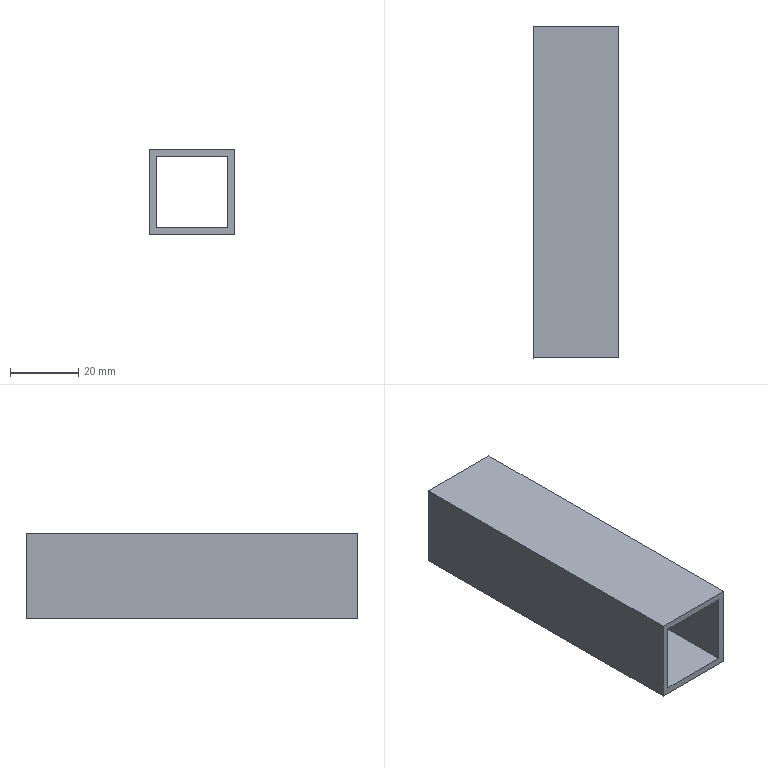Part | NX | features solid 2 | 1 solid | 10 faces | box 25 x 97 x 25 mm | volume 17848 mm3 | plane 10
STEP:
#1=CARTESIAN_POINT('',(-97.5,-106.5,-75.));
#2=VERTEX_POINT('',#1);
#3=CARTESIAN_POINT('',(-97.5,-203.5,-75.));
#4=VERTEX_POINT('',#3);
#5=CARTESIAN_POINT('',(-97.5,-125.,-75.));
#6=DIRECTION('',(0.,-1.,0.));
#7=VECTOR('',#6,1000.);
#8=LINE('',#5,#7);
#9=EDGE_CURVE('',#2,#4,#8,.T.);
#10=ORIENTED_EDGE('',*,*,#9,.T.);
#11=CARTESIAN_POINT('',(-122.5,-203.5,-75.));
#12=VERTEX_POINT('',#11);
#13=CARTESIAN_POINT('',(-95.,-203.5,-75.));
#14=DIRECTION('',(-1.,0.,0.));
#15=VECTOR('',#14,1000.);
#16=LINE('',#13,#15);
#17=EDGE_CURVE('',#4,#12,#16,.T.);
#18=ORIENTED_EDGE('',*,*,#17,.T.);
#19=CARTESIAN_POINT('',(-122.5,-106.5,-75.));
#20=VERTEX_POINT('',#19);
#21=CARTESIAN_POINT('',(-122.5,-125.,-75.));
#22=DIRECTION('',(0.,-1.,0.));
#23=VECTOR('',#22,1000.);
#24=LINE('',#21,#23);
#25=EDGE_CURVE('',#20,#12,#24,.T.);
#26=ORIENTED_EDGE('',*,*,#25,.F.);
#27=CARTESIAN_POINT('',(-95.,-106.5,-75.));
#28=DIRECTION('',(1.,0.,0.));
#29=VECTOR('',#28,1000.);
#30=LINE('',#27,#29);
#31=EDGE_CURVE('',#2,#20,#30,.F.);
#32=ORIENTED_EDGE('',*,*,#31,.F.);
#33=EDGE_LOOP('',(#10,#18,#26,#32));
#34=FACE_BOUND('',#33,.T.);
#35=CARTESIAN_POINT('',(-95.,-125.,-75.));
#36=DIRECTION('',(0.,0.,-1.));
#37=DIRECTION('',(-1.,0.,0.));
#38=AXIS2_PLACEMENT_3D('',#35,#36,#37);
#39=PLANE('',#38);
#40=ADVANCED_FACE('',(#34),#39,.T.);
#41=CARTESIAN_POINT('',(-97.5,-106.5,-50.));
#42=VERTEX_POINT('',#41);
#43=CARTESIAN_POINT('',(-97.5,-203.5,-50.));
#44=VERTEX_POINT('',#43);
#45=CARTESIAN_POINT('',(-97.5,-125.,-50.));
#46=DIRECTION('',(0.,-1.,0.));
#47=VECTOR('',#46,1000.);
#48=LINE('',#45,#47);
#49=EDGE_CURVE('',#42,#44,#48,.T.);
#50=ORIENTED_EDGE('',*,*,#49,.T.);
#51=CARTESIAN_POINT('',(-97.5,-203.5,-47.5));
#52=DIRECTION('',(0.,0.,-1.));
#53=VECTOR('',#52,1000.);
#54=LINE('',#51,#53);
#55=EDGE_CURVE('',#44,#4,#54,.T.);
#56=ORIENTED_EDGE('',*,*,#55,.T.);
#57=ORIENTED_EDGE('',*,*,#9,.F.);
#58=CARTESIAN_POINT('',(-97.5,-106.5,-47.5));
#59=DIRECTION('',(0.,0.,1.));
#60=VECTOR('',#59,1000.);
#61=LINE('',#58,#60);
#62=EDGE_CURVE('',#42,#2,#61,.F.);
#63=ORIENTED_EDGE('',*,*,#62,.F.);
#64=EDGE_LOOP('',(#50,#56,#57,#63));
#65=FACE_BOUND('',#64,.T.);
#66=CARTESIAN_POINT('',(-97.5,-125.,-47.5));
#67=DIRECTION('',(1.,0.,0.));
#68=DIRECTION('',(0.,0.,-1.));
#69=AXIS2_PLACEMENT_3D('',#66,#67,#68);
#70=PLANE('',#69);
#71=ADVANCED_FACE('',(#65),#70,.T.);
#72=CARTESIAN_POINT('',(-122.5,-106.5,-50.));
#73=VERTEX_POINT('',#72);
#74=CARTESIAN_POINT('',(-122.5,-203.5,-50.));
#75=VERTEX_POINT('',#74);
#76=CARTESIAN_POINT('',(-122.5,-125.,-50.));
#77=DIRECTION('',(0.,-1.,0.));
#78=VECTOR('',#77,1000.);
#79=LINE('',#76,#78);
#80=EDGE_CURVE('',#73,#75,#79,.T.);
#81=ORIENTED_EDGE('',*,*,#80,.T.);
#82=CARTESIAN_POINT('',(-125.,-203.5,-50.));
#83=DIRECTION('',(1.,0.,0.));
#84=VECTOR('',#83,1000.);
#85=LINE('',#82,#84);
#86=EDGE_CURVE('',#75,#44,#85,.T.);
#87=ORIENTED_EDGE('',*,*,#86,.T.);
#88=ORIENTED_EDGE('',*,*,#49,.F.);
#89=CARTESIAN_POINT('',(-125.,-106.5,-50.));
#90=DIRECTION('',(-1.,0.,0.));
#91=VECTOR('',#90,1000.);
#92=LINE('',#89,#91);
#93=EDGE_CURVE('',#73,#42,#92,.F.);
#94=ORIENTED_EDGE('',*,*,#93,.F.);
#95=EDGE_LOOP('',(#81,#87,#88,#94));
#96=FACE_BOUND('',#95,.T.);
#97=CARTESIAN_POINT('',(-125.,-125.,-50.));
#98=DIRECTION('',(0.,0.,1.));
#99=DIRECTION('',(1.,0.,0.));
#100=AXIS2_PLACEMENT_3D('',#97,#98,#99);
#101=PLANE('',#100);
#102=ADVANCED_FACE('',(#96),#101,.T.);
#103=ORIENTED_EDGE('',*,*,#25,.T.);
#104=CARTESIAN_POINT('',(-122.5,-203.5,-77.5));
#105=DIRECTION('',(0.,0.,1.));
#106=VECTOR('',#105,1000.);
#107=LINE('',#104,#106);
#108=EDGE_CURVE('',#12,#75,#107,.T.);
#109=ORIENTED_EDGE('',*,*,#108,.T.);
#110=ORIENTED_EDGE('',*,*,#80,.F.);
#111=CARTESIAN_POINT('',(-122.5,-106.5,-77.5));
#112=DIRECTION('',(0.,0.,-1.));
#113=VECTOR('',#112,1000.);
#114=LINE('',#111,#113);
#115=EDGE_CURVE('',#20,#73,#114,.F.);
#116=ORIENTED_EDGE('',*,*,#115,.F.);
#117=EDGE_LOOP('',(#103,#109,#110,#116));
#118=FACE_BOUND('',#117,.T.);
#119=CARTESIAN_POINT('',(-122.5,-125.,-77.5));
#120=DIRECTION('',(-1.,0.,0.));
#121=DIRECTION('',(0.,0.,1.));
#122=AXIS2_PLACEMENT_3D('',#119,#120,#121);
#123=PLANE('',#122);
#124=ADVANCED_FACE('',(#118),#123,.T.);
#125=CARTESIAN_POINT('',(-99.5,-106.5,-73.));
#126=VERTEX_POINT('',#125);
#127=CARTESIAN_POINT('',(-120.5,-106.5,-73.));
#128=VERTEX_POINT('',#127);
#129=CARTESIAN_POINT('',(-95.,-106.5,-73.));
#130=DIRECTION('',(1.,0.,0.));
#131=VECTOR('',#130,1000.);
#132=LINE('',#129,#131);
#133=EDGE_CURVE('',#126,#128,#132,.F.);
#134=ORIENTED_EDGE('',*,*,#133,.T.);
#135=CARTESIAN_POINT('',(-120.5,-203.5,-73.));
#136=VERTEX_POINT('',#135);
#137=CARTESIAN_POINT('',(-120.5,-125.,-73.));
#138=DIRECTION('',(0.,-1.,0.));
#139=VECTOR('',#138,1000.);
#140=LINE('',#137,#139);
#141=EDGE_CURVE('',#128,#136,#140,.T.);
#142=ORIENTED_EDGE('',*,*,#141,.T.);
#143=CARTESIAN_POINT('',(-99.5,-203.5,-73.));
#144=VERTEX_POINT('',#143);
#145=CARTESIAN_POINT('',(-95.,-203.5,-73.));
#146=DIRECTION('',(-1.,0.,0.));
#147=VECTOR('',#146,1000.);
#148=LINE('',#145,#147);
#149=EDGE_CURVE('',#144,#136,#148,.T.);
#150=ORIENTED_EDGE('',*,*,#149,.F.);
#151=CARTESIAN_POINT('',(-99.5,-125.,-73.));
#152=DIRECTION('',(0.,-1.,0.));
#153=VECTOR('',#152,1000.);
#154=LINE('',#151,#153);
#155=EDGE_CURVE('',#126,#144,#154,.T.);
#156=ORIENTED_EDGE('',*,*,#155,.F.);
#157=EDGE_LOOP('',(#134,#142,#150,#156));
#158=FACE_BOUND('',#157,.T.);
#159=CARTESIAN_POINT('',(-95.,-125.,-73.));
#160=DIRECTION('',(0.,0.,-1.));
#161=DIRECTION('',(-1.,0.,0.));
#162=AXIS2_PLACEMENT_3D('',#159,#160,#161);
#163=PLANE('',#162);
#164=ADVANCED_FACE('',(#158),#163,.F.);
#165=CARTESIAN_POINT('',(-99.5,-106.5,-52.));
#166=VERTEX_POINT('',#165);
#167=CARTESIAN_POINT('',(-99.5,-106.5,-47.5));
#168=DIRECTION('',(0.,0.,1.));
#169=VECTOR('',#168,1000.);
#170=LINE('',#167,#169);
#171=EDGE_CURVE('',#166,#126,#170,.F.);
#172=ORIENTED_EDGE('',*,*,#171,.T.);
#173=ORIENTED_EDGE('',*,*,#155,.T.);
#174=CARTESIAN_POINT('',(-99.5,-203.5,-52.));
#175=VERTEX_POINT('',#174);
#176=CARTESIAN_POINT('',(-99.5,-203.5,-47.5));
#177=DIRECTION('',(0.,0.,-1.));
#178=VECTOR('',#177,1000.);
#179=LINE('',#176,#178);
#180=EDGE_CURVE('',#175,#144,#179,.T.);
#181=ORIENTED_EDGE('',*,*,#180,.F.);
#182=CARTESIAN_POINT('',(-99.5,-125.,-52.));
#183=DIRECTION('',(0.,-1.,0.));
#184=VECTOR('',#183,1000.);
#185=LINE('',#182,#184);
#186=EDGE_CURVE('',#166,#175,#185,.T.);
#187=ORIENTED_EDGE('',*,*,#186,.F.);
#188=EDGE_LOOP('',(#172,#173,#181,#187));
#189=FACE_BOUND('',#188,.T.);
#190=CARTESIAN_POINT('',(-99.5,-125.,-47.5));
#191=DIRECTION('',(1.,0.,0.));
#192=DIRECTION('',(0.,0.,-1.));
#193=AXIS2_PLACEMENT_3D('',#190,#191,#192);
#194=PLANE('',#193);
#195=ADVANCED_FACE('',(#189),#194,.F.);
#196=CARTESIAN_POINT('',(-120.5,-106.5,-52.));
#197=VERTEX_POINT('',#196);
#198=CARTESIAN_POINT('',(-125.,-106.5,-52.));
#199=DIRECTION('',(-1.,0.,0.));
#200=VECTOR('',#199,1000.);
#201=LINE('',#198,#200);
#202=EDGE_CURVE('',#197,#166,#201,.F.);
#203=ORIENTED_EDGE('',*,*,#202,.T.);
#204=ORIENTED_EDGE('',*,*,#186,.T.);
#205=CARTESIAN_POINT('',(-120.5,-203.5,-52.));
#206=VERTEX_POINT('',#205);
#207=CARTESIAN_POINT('',(-125.,-203.5,-52.));
#208=DIRECTION('',(1.,0.,0.));
#209=VECTOR('',#208,1000.);
#210=LINE('',#207,#209);
#211=EDGE_CURVE('',#206,#175,#210,.T.);
#212=ORIENTED_EDGE('',*,*,#211,.F.);
#213=CARTESIAN_POINT('',(-120.5,-125.,-52.));
#214=DIRECTION('',(0.,-1.,0.));
#215=VECTOR('',#214,1000.);
#216=LINE('',#213,#215);
#217=EDGE_CURVE('',#197,#206,#216,.T.);
#218=ORIENTED_EDGE('',*,*,#217,.F.);
#219=EDGE_LOOP('',(#203,#204,#212,#218));
#220=FACE_BOUND('',#219,.T.);
#221=CARTESIAN_POINT('',(-125.,-125.,-52.));
#222=DIRECTION('',(0.,0.,1.));
#223=DIRECTION('',(1.,0.,0.));
#224=AXIS2_PLACEMENT_3D('',#221,#222,#223);
#225=PLANE('',#224);
#226=ADVANCED_FACE('',(#220),#225,.F.);
#227=CARTESIAN_POINT('',(-120.5,-106.5,-77.5));
#228=DIRECTION('',(0.,0.,-1.));
#229=VECTOR('',#228,1000.);
#230=LINE('',#227,#229);
#231=EDGE_CURVE('',#128,#197,#230,.F.);
#232=ORIENTED_EDGE('',*,*,#231,.T.);
#233=ORIENTED_EDGE('',*,*,#217,.T.);
#234=CARTESIAN_POINT('',(-120.5,-203.5,-77.5));
#235=DIRECTION('',(0.,0.,1.));
#236=VECTOR('',#235,1000.);
#237=LINE('',#234,#236);
#238=EDGE_CURVE('',#136,#206,#237,.T.);
#239=ORIENTED_EDGE('',*,*,#238,.F.);
#240=ORIENTED_EDGE('',*,*,#141,.F.);
#241=EDGE_LOOP('',(#232,#233,#239,#240));
#242=FACE_BOUND('',#241,.T.);
#243=CARTESIAN_POINT('',(-120.5,-125.,-77.5));
#244=DIRECTION('',(-1.,0.,0.));
#245=DIRECTION('',(0.,0.,1.));
#246=AXIS2_PLACEMENT_3D('',#243,#244,#245);
#247=PLANE('',#246);
#248=ADVANCED_FACE('',(#242),#247,.F.);
#249=ORIENTED_EDGE('',*,*,#108,.F.);
#250=ORIENTED_EDGE('',*,*,#17,.F.);
#251=ORIENTED_EDGE('',*,*,#55,.F.);
#252=ORIENTED_EDGE('',*,*,#86,.F.);
#253=EDGE_LOOP('',(#249,#250,#251,#252));
#254=FACE_BOUND('',#253,.T.);
#255=ORIENTED_EDGE('',*,*,#149,.T.);
#256=ORIENTED_EDGE('',*,*,#238,.T.);
#257=ORIENTED_EDGE('',*,*,#211,.T.);
#258=ORIENTED_EDGE('',*,*,#180,.T.);
#259=EDGE_LOOP('',(#255,#256,#257,#258));
#260=FACE_BOUND('',#259,.T.);
#261=CARTESIAN_POINT('',(94.,-203.5,-77.5));
#262=DIRECTION('',(0.,1.,0.));
#263=DIRECTION('',(0.,0.,1.));
#264=AXIS2_PLACEMENT_3D('',#261,#262,#263);
#265=PLANE('',#264);
#266=ADVANCED_FACE('',(#254,#260),#265,.F.);
#267=ORIENTED_EDGE('',*,*,#31,.T.);
#268=ORIENTED_EDGE('',*,*,#115,.T.);
#269=ORIENTED_EDGE('',*,*,#93,.T.);
#270=ORIENTED_EDGE('',*,*,#62,.T.);
#271=EDGE_LOOP('',(#267,#268,#269,#270));
#272=FACE_BOUND('',#271,.T.);
#273=ORIENTED_EDGE('',*,*,#171,.F.);
#274=ORIENTED_EDGE('',*,*,#202,.F.);
#275=ORIENTED_EDGE('',*,*,#231,.F.);
#276=ORIENTED_EDGE('',*,*,#133,.F.);
#277=EDGE_LOOP('',(#273,#274,#275,#276));
#278=FACE_BOUND('',#277,.T.);
#279=CARTESIAN_POINT('',(-94.,-106.5,-47.5));
#280=DIRECTION('',(0.,-1.,0.));
#281=DIRECTION('',(0.,0.,-1.));
#282=AXIS2_PLACEMENT_3D('',#279,#280,#281);
#283=PLANE('',#282);
#284=ADVANCED_FACE('',(#272,#278),#283,.F.);
#285=CLOSED_SHELL('',(#40,#71,#102,#124,#164,#195,#226,#248,#266,#284));
#286=MANIFOLD_SOLID_BREP('',#285);
#287=(LENGTH_UNIT()NAMED_UNIT(*)SI_UNIT(.MILLI.,.METRE.));
#288=UNCERTAINTY_MEASURE_WITH_UNIT(LENGTH_MEASURE(0.00001),#287,'','');
#289=(NAMED_UNIT(*)PLANE_ANGLE_UNIT()SI_UNIT($,.RADIAN.));
#290=(NAMED_UNIT(*)SI_UNIT($,.STERADIAN.)SOLID_ANGLE_UNIT());
#291=(GEOMETRIC_REPRESENTATION_CONTEXT(3)GLOBAL_UNCERTAINTY_ASSIGNED_CONTEXT((#288))GLOBAL_UNIT_ASSIGNED_CONTEXT((#287,#289,#290))REPRESENTATION_CONTEXT('',''));
#292=ADVANCED_BREP_SHAPE_REPRESENTATION('',(#286),#291);